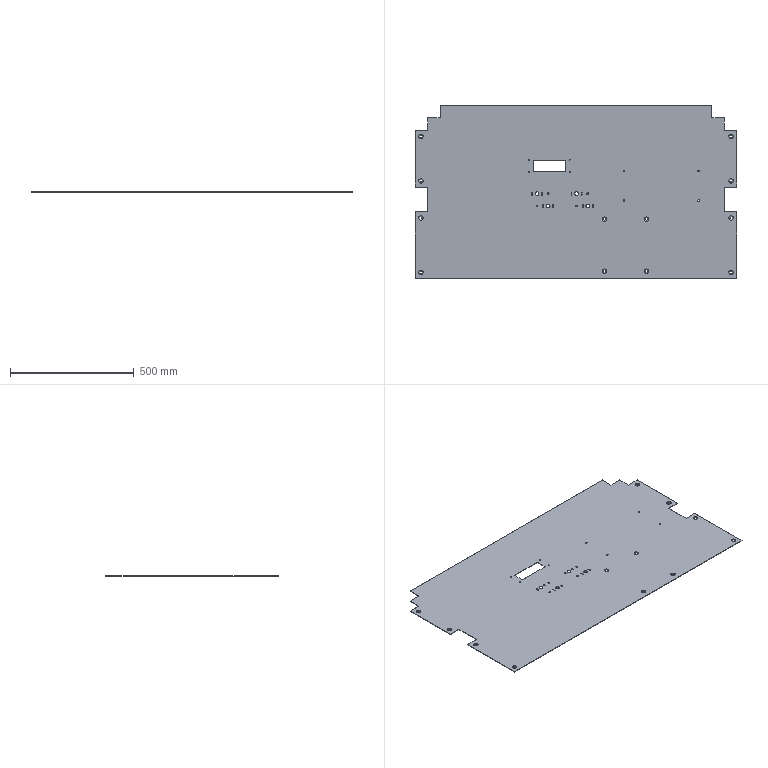Part | STEP file | 1300 table 1 | 1 solid | 114 faces | box 1300 x 700 x 2 mm | volume 1751949 mm3 | cylinder 64 | plane 26 | cone 24 | commonest cylinder face diameters 3.3 x40 6.8 x16 15 x8